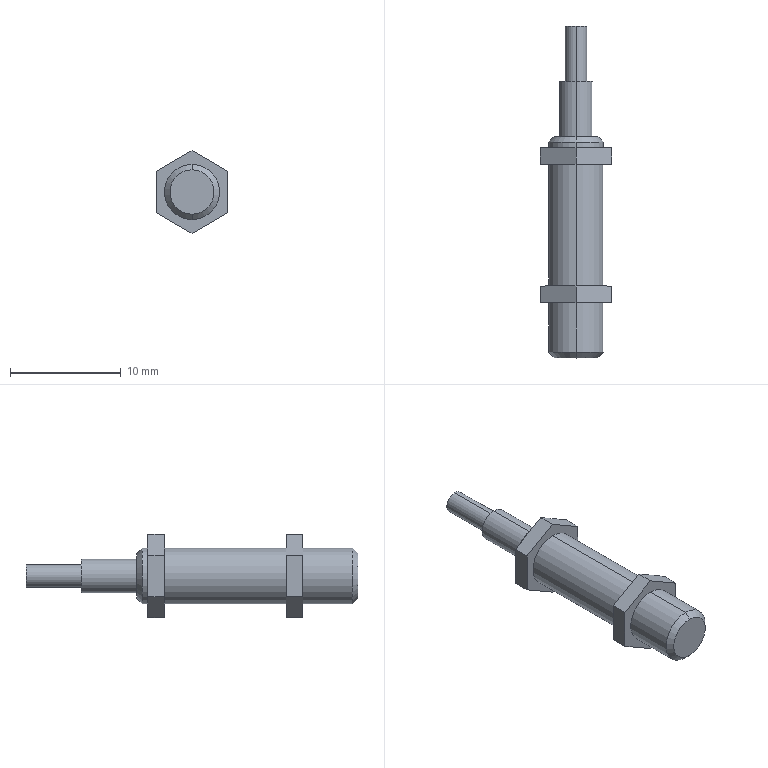Part | STEP file | Guide wheel mechanism revised.sldasm-Part-49 | 1 solid | 34 faces | box 6.5 x 30 x 7.506 mm | volume 490.949 mm3 | plane 20 | cylinder 10 | cone 4 | commonest cylinder face diameters 5 x6 2 x2 3 x2
STEP:
#1=CARTESIAN_POINT('',(0.,17.5,-2.5));
#2=VERTEX_POINT('',#1);
#3=CARTESIAN_POINT('',(0.,17.5,2.5));
#4=VERTEX_POINT('',#3);
#5=CARTESIAN_POINT('',(0.,17.5,0.));
#6=DIRECTION('',(0.,-1.,0.));
#7=DIRECTION('',(0.,0.,-1.));
#8=AXIS2_PLACEMENT_3D('',#5,#6,#7);
#9=CIRCLE('',#8,2.5);
#10=EDGE_CURVE('',#2,#4,#9,.T.);
#11=ORIENTED_EDGE('',*,*,#10,.T.);
#12=CARTESIAN_POINT('',(0.,6.5,2.5));
#13=VERTEX_POINT('',#12);
#14=CARTESIAN_POINT('',(0.,20.,2.5));
#15=DIRECTION('',(0.,-1.,0.));
#16=VECTOR('',#15,1000.);
#17=LINE('',#14,#16);
#18=EDGE_CURVE('',#4,#13,#17,.T.);
#19=ORIENTED_EDGE('',*,*,#18,.T.);
#20=CARTESIAN_POINT('',(0.,6.5,-2.5));
#21=VERTEX_POINT('',#20);
#22=CARTESIAN_POINT('',(0.,6.5,0.));
#23=DIRECTION('',(0.,-1.,0.));
#24=DIRECTION('',(0.,0.,-1.));
#25=AXIS2_PLACEMENT_3D('',#22,#23,#24);
#26=CIRCLE('',#25,2.5);
#27=EDGE_CURVE('',#21,#13,#26,.T.);
#28=ORIENTED_EDGE('',*,*,#27,.F.);
#29=CARTESIAN_POINT('',(0.,20.,-2.5));
#30=DIRECTION('',(0.,-1.,0.));
#31=VECTOR('',#30,1000.);
#32=LINE('',#29,#31);
#33=EDGE_CURVE('',#2,#21,#32,.T.);
#34=ORIENTED_EDGE('',*,*,#33,.F.);
#35=EDGE_LOOP('',(#11,#19,#28,#34));
#36=FACE_OUTER_BOUND('',#35,.T.);
#37=CARTESIAN_POINT('',(0.,20.,0.));
#38=DIRECTION('',(0.,-1.,0.));
#39=DIRECTION('',(0.,0.,-1.));
#40=AXIS2_PLACEMENT_3D('',#37,#38,#39);
#41=CYLINDRICAL_SURFACE('',#40,2.5);
#42=ADVANCED_FACE('',(#36),#41,.T.);
#43=CARTESIAN_POINT('',(0.,5.,-2.5));
#44=VERTEX_POINT('',#43);
#45=CARTESIAN_POINT('',(0.,5.,2.5));
#46=VERTEX_POINT('',#45);
#47=CARTESIAN_POINT('',(0.,5.,0.));
#48=DIRECTION('',(0.,-1.,0.));
#49=DIRECTION('',(0.,0.,-1.));
#50=AXIS2_PLACEMENT_3D('',#47,#48,#49);
#51=CIRCLE('',#50,2.5);
#52=EDGE_CURVE('',#44,#46,#51,.T.);
#53=ORIENTED_EDGE('',*,*,#52,.T.);
#54=CARTESIAN_POINT('',(0.,0.5,2.5));
#55=VERTEX_POINT('',#54);
#56=CARTESIAN_POINT('',(0.,20.,2.5));
#57=DIRECTION('',(0.,-1.,0.));
#58=VECTOR('',#57,1000.);
#59=LINE('',#56,#58);
#60=EDGE_CURVE('',#46,#55,#59,.T.);
#61=ORIENTED_EDGE('',*,*,#60,.T.);
#62=CARTESIAN_POINT('',(0.,0.5,-2.5));
#63=VERTEX_POINT('',#62);
#64=CARTESIAN_POINT('',(0.,0.5,0.));
#65=DIRECTION('',(0.,1.,0.));
#66=DIRECTION('',(0.,0.,1.));
#67=AXIS2_PLACEMENT_3D('',#64,#65,#66);
#68=CIRCLE('',#67,2.5);
#69=EDGE_CURVE('',#55,#63,#68,.T.);
#70=ORIENTED_EDGE('',*,*,#69,.T.);
#71=CARTESIAN_POINT('',(0.,20.,-2.5));
#72=DIRECTION('',(0.,-1.,0.));
#73=VECTOR('',#72,1000.);
#74=LINE('',#71,#73);
#75=EDGE_CURVE('',#44,#63,#74,.T.);
#76=ORIENTED_EDGE('',*,*,#75,.F.);
#77=EDGE_LOOP('',(#53,#61,#70,#76));
#78=FACE_OUTER_BOUND('',#77,.T.);
#79=CARTESIAN_POINT('',(0.,20.,0.));
#80=DIRECTION('',(0.,-1.,0.));
#81=DIRECTION('',(0.,0.,-1.));
#82=AXIS2_PLACEMENT_3D('',#79,#80,#81);
#83=CYLINDRICAL_SURFACE('',#82,2.5);
#84=ADVANCED_FACE('',(#78),#83,.T.);
#85=CARTESIAN_POINT('',(0.,0.,-2.));
#86=VERTEX_POINT('',#85);
#87=CARTESIAN_POINT('',(0.,0.,2.));
#88=VERTEX_POINT('',#87);
#89=CARTESIAN_POINT('',(0.,0.,0.));
#90=DIRECTION('',(0.,-1.,0.));
#91=DIRECTION('',(0.,0.,1.));
#92=AXIS2_PLACEMENT_3D('',#89,#90,#91);
#93=CIRCLE('',#92,2.);
#94=EDGE_CURVE('',#86,#88,#93,.T.);
#95=ORIENTED_EDGE('',*,*,#94,.F.);
#96=CARTESIAN_POINT('',(0.,0.5,-2.5));
#97=DIRECTION('',(0.,0.7071,-0.7071));
#98=VECTOR('',#97,1000.);
#99=LINE('',#96,#98);
#100=EDGE_CURVE('',#86,#63,#99,.T.);
#101=ORIENTED_EDGE('',*,*,#100,.T.);
#102=ORIENTED_EDGE('',*,*,#69,.F.);
#103=CARTESIAN_POINT('',(0.,0.5,2.5));
#104=DIRECTION('',(0.,0.7071,0.7071));
#105=VECTOR('',#104,1000.);
#106=LINE('',#103,#105);
#107=EDGE_CURVE('',#88,#55,#106,.T.);
#108=ORIENTED_EDGE('',*,*,#107,.F.);
#109=EDGE_LOOP('',(#95,#101,#102,#108));
#110=FACE_OUTER_BOUND('',#109,.T.);
#111=CARTESIAN_POINT('',(0.,0.5,0.));
#112=DIRECTION('',(0.,1.,0.));
#113=DIRECTION('',(0.,0.,1.));
#114=AXIS2_PLACEMENT_3D('',#111,#112,#113);
#115=CONICAL_SURFACE('',#114,2.5,0.7854);
#116=ADVANCED_FACE('',(#110),#115,.T.);
#117=CARTESIAN_POINT('',(0.,30.,1.));
#118=VERTEX_POINT('',#117);
#119=CARTESIAN_POINT('',(0.,30.,-1.));
#120=VERTEX_POINT('',#119);
#121=CARTESIAN_POINT('',(0.,30.,0.));
#122=DIRECTION('',(0.,1.,0.));
#123=DIRECTION('',(0.,0.,1.));
#124=AXIS2_PLACEMENT_3D('',#121,#122,#123);
#125=CIRCLE('',#124,1.);
#126=EDGE_CURVE('',#118,#120,#125,.T.);
#127=ORIENTED_EDGE('',*,*,#126,.F.);
#128=CARTESIAN_POINT('',(0.,25.,1.));
#129=VERTEX_POINT('',#128);
#130=CARTESIAN_POINT('',(0.,30.,1.));
#131=DIRECTION('',(0.,-1.,0.));
#132=VECTOR('',#131,1000.);
#133=LINE('',#130,#132);
#134=EDGE_CURVE('',#118,#129,#133,.T.);
#135=ORIENTED_EDGE('',*,*,#134,.T.);
#136=CARTESIAN_POINT('',(0.,25.,-1.));
#137=VERTEX_POINT('',#136);
#138=CARTESIAN_POINT('',(0.,25.,0.));
#139=DIRECTION('',(0.,1.,0.));
#140=DIRECTION('',(0.,0.,1.));
#141=AXIS2_PLACEMENT_3D('',#138,#139,#140);
#142=CIRCLE('',#141,1.);
#143=EDGE_CURVE('',#129,#137,#142,.T.);
#144=ORIENTED_EDGE('',*,*,#143,.T.);
#145=CARTESIAN_POINT('',(0.,30.,-1.));
#146=DIRECTION('',(0.,-1.,0.));
#147=VECTOR('',#146,1000.);
#148=LINE('',#145,#147);
#149=EDGE_CURVE('',#120,#137,#148,.T.);
#150=ORIENTED_EDGE('',*,*,#149,.F.);
#151=EDGE_LOOP('',(#127,#135,#144,#150));
#152=FACE_OUTER_BOUND('',#151,.T.);
#153=CARTESIAN_POINT('',(0.,30.,0.));
#154=DIRECTION('',(0.,-1.,0.));
#155=DIRECTION('',(0.,0.,-1.));
#156=AXIS2_PLACEMENT_3D('',#153,#154,#155);
#157=CYLINDRICAL_SURFACE('',#156,1.);
#158=ADVANCED_FACE('',(#152),#157,.T.);
#159=CARTESIAN_POINT('',(0.,25.,1.5));
#160=VERTEX_POINT('',#159);
#161=CARTESIAN_POINT('',(0.,25.,-1.5));
#162=VERTEX_POINT('',#161);
#163=CARTESIAN_POINT('',(0.,25.,0.));
#164=DIRECTION('',(0.,1.,0.));
#165=DIRECTION('',(0.,0.,1.));
#166=AXIS2_PLACEMENT_3D('',#163,#164,#165);
#167=CIRCLE('',#166,1.5);
#168=EDGE_CURVE('',#160,#162,#167,.T.);
#169=ORIENTED_EDGE('',*,*,#168,.F.);
#170=CARTESIAN_POINT('',(0.,20.,1.5));
#171=VERTEX_POINT('',#170);
#172=CARTESIAN_POINT('',(0.,25.,1.5));
#173=DIRECTION('',(0.,-1.,0.));
#174=VECTOR('',#173,1000.);
#175=LINE('',#172,#174);
#176=EDGE_CURVE('',#160,#171,#175,.T.);
#177=ORIENTED_EDGE('',*,*,#176,.T.);
#178=CARTESIAN_POINT('',(0.,20.,-1.5));
#179=VERTEX_POINT('',#178);
#180=CARTESIAN_POINT('',(0.,20.,0.));
#181=DIRECTION('',(0.,1.,0.));
#182=DIRECTION('',(0.,0.,1.));
#183=AXIS2_PLACEMENT_3D('',#180,#181,#182);
#184=CIRCLE('',#183,1.5);
#185=EDGE_CURVE('',#171,#179,#184,.T.);
#186=ORIENTED_EDGE('',*,*,#185,.T.);
#187=CARTESIAN_POINT('',(0.,25.,-1.5));
#188=DIRECTION('',(0.,-1.,0.));
#189=VECTOR('',#188,1000.);
#190=LINE('',#187,#189);
#191=EDGE_CURVE('',#162,#179,#190,.T.);
#192=ORIENTED_EDGE('',*,*,#191,.F.);
#193=EDGE_LOOP('',(#169,#177,#186,#192));
#194=FACE_OUTER_BOUND('',#193,.T.);
#195=CARTESIAN_POINT('',(0.,25.,0.));
#196=DIRECTION('',(0.,-1.,0.));
#197=DIRECTION('',(0.,0.,-1.));
#198=AXIS2_PLACEMENT_3D('',#195,#196,#197);
#199=CYLINDRICAL_SURFACE('',#198,1.5);
#200=ADVANCED_FACE('',(#194),#199,.T.);
#201=CARTESIAN_POINT('',(0.,20.,2.));
#202=VERTEX_POINT('',#201);
#203=CARTESIAN_POINT('',(0.,20.,-2.));
#204=VERTEX_POINT('',#203);
#205=CARTESIAN_POINT('',(0.,20.,0.));
#206=DIRECTION('',(0.,1.,0.));
#207=DIRECTION('',(0.,0.,1.));
#208=AXIS2_PLACEMENT_3D('',#205,#206,#207);
#209=CIRCLE('',#208,2.);
#210=EDGE_CURVE('',#202,#204,#209,.T.);
#211=ORIENTED_EDGE('',*,*,#210,.F.);
#212=CARTESIAN_POINT('',(0.,19.5,2.5));
#213=VERTEX_POINT('',#212);
#214=CARTESIAN_POINT('',(0.,20.,2.));
#215=DIRECTION('',(0.,-0.7071,0.7071));
#216=VECTOR('',#215,1000.);
#217=LINE('',#214,#216);
#218=EDGE_CURVE('',#202,#213,#217,.T.);
#219=ORIENTED_EDGE('',*,*,#218,.T.);
#220=CARTESIAN_POINT('',(0.,19.5,-2.5));
#221=VERTEX_POINT('',#220);
#222=CARTESIAN_POINT('',(0.,19.5,0.));
#223=DIRECTION('',(0.,-1.,0.));
#224=DIRECTION('',(0.,0.,1.));
#225=AXIS2_PLACEMENT_3D('',#222,#223,#224);
#226=CIRCLE('',#225,2.5);
#227=EDGE_CURVE('',#221,#213,#226,.T.);
#228=ORIENTED_EDGE('',*,*,#227,.F.);
#229=CARTESIAN_POINT('',(0.,20.,-2.));
#230=DIRECTION('',(0.,-0.7071,-0.7071));
#231=VECTOR('',#230,1000.);
#232=LINE('',#229,#231);
#233=EDGE_CURVE('',#204,#221,#232,.T.);
#234=ORIENTED_EDGE('',*,*,#233,.F.);
#235=EDGE_LOOP('',(#211,#219,#228,#234));
#236=FACE_OUTER_BOUND('',#235,.T.);
#237=CARTESIAN_POINT('',(0.,20.,0.));
#238=DIRECTION('',(0.,-1.,0.));
#239=DIRECTION('',(0.,0.,-1.));
#240=AXIS2_PLACEMENT_3D('',#237,#238,#239);
#241=CONICAL_SURFACE('',#240,2.,0.7854);
#242=ADVANCED_FACE('',(#236),#241,.T.);
#243=ORIENTED_EDGE('',*,*,#227,.T.);
#244=CARTESIAN_POINT('',(0.,19.,2.5));
#245=VERTEX_POINT('',#244);
#246=CARTESIAN_POINT('',(0.,20.,2.5));
#247=DIRECTION('',(0.,-1.,0.));
#248=VECTOR('',#247,1000.);
#249=LINE('',#246,#248);
#250=EDGE_CURVE('',#213,#245,#249,.T.);
#251=ORIENTED_EDGE('',*,*,#250,.T.);
#252=CARTESIAN_POINT('',(0.,19.,-2.5));
#253=VERTEX_POINT('',#252);
#254=CARTESIAN_POINT('',(0.,19.,0.));
#255=DIRECTION('',(0.,-1.,0.));
#256=DIRECTION('',(0.,0.,-1.));
#257=AXIS2_PLACEMENT_3D('',#254,#255,#256);
#258=CIRCLE('',#257,2.5);
#259=EDGE_CURVE('',#253,#245,#258,.T.);
#260=ORIENTED_EDGE('',*,*,#259,.F.);
#261=CARTESIAN_POINT('',(0.,20.,-2.5));
#262=DIRECTION('',(0.,-1.,0.));
#263=VECTOR('',#262,1000.);
#264=LINE('',#261,#263);
#265=EDGE_CURVE('',#221,#253,#264,.T.);
#266=ORIENTED_EDGE('',*,*,#265,.F.);
#267=EDGE_LOOP('',(#243,#251,#260,#266));
#268=FACE_OUTER_BOUND('',#267,.T.);
#269=CARTESIAN_POINT('',(0.,20.,0.));
#270=DIRECTION('',(0.,-1.,0.));
#271=DIRECTION('',(0.,0.,-1.));
#272=AXIS2_PLACEMENT_3D('',#269,#270,#271);
#273=CYLINDRICAL_SURFACE('',#272,2.5);
#274=ADVANCED_FACE('',(#268),#273,.T.);
#275=ORIENTED_EDGE('',*,*,#250,.F.);
#276=CARTESIAN_POINT('',(0.,19.5,0.));
#277=DIRECTION('',(0.,-1.,0.));
#278=DIRECTION('',(0.,0.,1.));
#279=AXIS2_PLACEMENT_3D('',#276,#277,#278);
#280=CIRCLE('',#279,2.5);
#281=EDGE_CURVE('',#213,#221,#280,.T.);
#282=ORIENTED_EDGE('',*,*,#281,.T.);
#283=ORIENTED_EDGE('',*,*,#265,.T.);
#284=CARTESIAN_POINT('',(0.,19.,0.));
#285=DIRECTION('',(0.,-1.,0.));
#286=DIRECTION('',(0.,0.,-1.));
#287=AXIS2_PLACEMENT_3D('',#284,#285,#286);
#288=CIRCLE('',#287,2.5);
#289=EDGE_CURVE('',#245,#253,#288,.T.);
#290=ORIENTED_EDGE('',*,*,#289,.F.);
#291=EDGE_LOOP('',(#275,#282,#283,#290));
#292=FACE_OUTER_BOUND('',#291,.T.);
#293=CARTESIAN_POINT('',(0.,20.,0.));
#294=DIRECTION('',(0.,-1.,0.));
#295=DIRECTION('',(0.,0.,-1.));
#296=AXIS2_PLACEMENT_3D('',#293,#294,#295);
#297=CYLINDRICAL_SURFACE('',#296,2.5);
#298=ADVANCED_FACE('',(#292),#297,.T.);
#299=CARTESIAN_POINT('',(0.,25.,0.));
#300=DIRECTION('',(0.,1.,0.));
#301=DIRECTION('',(0.,0.,1.));
#302=AXIS2_PLACEMENT_3D('',#299,#300,#301);
#303=CIRCLE('',#302,1.5);
#304=EDGE_CURVE('',#162,#160,#303,.T.);
#305=ORIENTED_EDGE('',*,*,#304,.T.);
#306=ORIENTED_EDGE('',*,*,#168,.T.);
#307=EDGE_LOOP('',(#305,#306));
#308=FACE_OUTER_BOUND('',#307,.T.);
#309=CARTESIAN_POINT('',(0.,25.,0.));
#310=DIRECTION('',(0.,1.,0.));
#311=DIRECTION('',(0.,0.,1.));
#312=AXIS2_PLACEMENT_3D('',#309,#310,#311);
#313=CIRCLE('',#312,1.);
#314=EDGE_CURVE('',#137,#129,#313,.T.);
#315=ORIENTED_EDGE('',*,*,#314,.F.);
#316=ORIENTED_EDGE('',*,*,#143,.F.);
#317=EDGE_LOOP('',(#315,#316));
#318=FACE_BOUND('',#317,.T.);
#319=CARTESIAN_POINT('',(0.,25.,0.));
#320=DIRECTION('',(0.,1.,0.));
#321=DIRECTION('',(0.,0.,1.));
#322=AXIS2_PLACEMENT_3D('',#319,#320,#321);
#323=PLANE('',#322);
#324=ADVANCED_FACE('',(#308,#318),#323,.T.);
#325=CARTESIAN_POINT('',(0.,20.,0.));
#326=DIRECTION('',(0.,1.,0.));
#327=DIRECTION('',(0.,0.,1.));
#328=AXIS2_PLACEMENT_3D('',#325,#326,#327);
#329=CIRCLE('',#328,2.);
#330=EDGE_CURVE('',#204,#202,#329,.T.);
#331=ORIENTED_EDGE('',*,*,#330,.T.);
#332=ORIENTED_EDGE('',*,*,#210,.T.);
#333=EDGE_LOOP('',(#331,#332));
#334=FACE_OUTER_BOUND('',#333,.T.);
#335=CARTESIAN_POINT('',(0.,20.,0.));
#336=DIRECTION('',(0.,1.,0.));
#337=DIRECTION('',(0.,0.,1.));
#338=AXIS2_PLACEMENT_3D('',#335,#336,#337);
#339=CIRCLE('',#338,1.5);
#340=EDGE_CURVE('',#179,#171,#339,.T.);
#341=ORIENTED_EDGE('',*,*,#340,.F.);
#342=ORIENTED_EDGE('',*,*,#185,.F.);
#343=EDGE_LOOP('',(#341,#342));
#344=FACE_BOUND('',#343,.T.);
#345=CARTESIAN_POINT('',(0.,20.,0.));
#346=DIRECTION('',(0.,1.,0.));
#347=DIRECTION('',(0.,0.,1.));
#348=AXIS2_PLACEMENT_3D('',#345,#346,#347);
#349=PLANE('',#348);
#350=ADVANCED_FACE('',(#334,#344),#349,.T.);
#351=ORIENTED_EDGE('',*,*,#218,.F.);
#352=ORIENTED_EDGE('',*,*,#330,.F.);
#353=ORIENTED_EDGE('',*,*,#233,.T.);
#354=ORIENTED_EDGE('',*,*,#281,.F.);
#355=EDGE_LOOP('',(#351,#352,#353,#354));
#356=FACE_OUTER_BOUND('',#355,.T.);
#357=CARTESIAN_POINT('',(0.,20.,0.));
#358=DIRECTION('',(0.,-1.,0.));
#359=DIRECTION('',(0.,0.,-1.));
#360=AXIS2_PLACEMENT_3D('',#357,#358,#359);
#361=CONICAL_SURFACE('',#360,2.,0.7854);
#362=ADVANCED_FACE('',(#356),#361,.T.);
#363=ORIENTED_EDGE('',*,*,#176,.F.);
#364=ORIENTED_EDGE('',*,*,#304,.F.);
#365=ORIENTED_EDGE('',*,*,#191,.T.);
#366=ORIENTED_EDGE('',*,*,#340,.T.);
#367=EDGE_LOOP('',(#363,#364,#365,#366));
#368=FACE_OUTER_BOUND('',#367,.T.);
#369=CARTESIAN_POINT('',(0.,25.,0.));
#370=DIRECTION('',(0.,-1.,0.));
#371=DIRECTION('',(0.,0.,-1.));
#372=AXIS2_PLACEMENT_3D('',#369,#370,#371);
#373=CYLINDRICAL_SURFACE('',#372,1.5);
#374=ADVANCED_FACE('',(#368),#373,.T.);
#375=ORIENTED_EDGE('',*,*,#134,.F.);
#376=CARTESIAN_POINT('',(0.,30.,0.));
#377=DIRECTION('',(0.,1.,0.));
#378=DIRECTION('',(0.,0.,1.));
#379=AXIS2_PLACEMENT_3D('',#376,#377,#378);
#380=CIRCLE('',#379,1.);
#381=EDGE_CURVE('',#120,#118,#380,.T.);
#382=ORIENTED_EDGE('',*,*,#381,.F.);
#383=ORIENTED_EDGE('',*,*,#149,.T.);
#384=ORIENTED_EDGE('',*,*,#314,.T.);
#385=EDGE_LOOP('',(#375,#382,#383,#384));
#386=FACE_OUTER_BOUND('',#385,.T.);
#387=CARTESIAN_POINT('',(0.,30.,0.));
#388=DIRECTION('',(0.,-1.,0.));
#389=DIRECTION('',(0.,0.,-1.));
#390=AXIS2_PLACEMENT_3D('',#387,#388,#389);
#391=CYLINDRICAL_SURFACE('',#390,1.);
#392=ADVANCED_FACE('',(#386),#391,.T.);
#393=ORIENTED_EDGE('',*,*,#381,.T.);
#394=ORIENTED_EDGE('',*,*,#126,.T.);
#395=EDGE_LOOP('',(#393,#394));
#396=FACE_OUTER_BOUND('',#395,.T.);
#397=CARTESIAN_POINT('',(0.,30.,0.));
#398=DIRECTION('',(0.,1.,0.));
#399=DIRECTION('',(0.,0.,1.));
#400=AXIS2_PLACEMENT_3D('',#397,#398,#399);
#401=PLANE('',#400);
#402=ADVANCED_FACE('',(#396),#401,.T.);
#403=CARTESIAN_POINT('',(3.25,17.5,1.876));
#404=VERTEX_POINT('',#403);
#405=CARTESIAN_POINT('',(0.,17.5,3.753));
#406=VERTEX_POINT('',#405);
#407=CARTESIAN_POINT('',(3.25,17.5,1.876));
#408=DIRECTION('',(-0.866,0.,0.5));
#409=VECTOR('',#408,1000.);
#410=LINE('',#407,#409);
#411=EDGE_CURVE('',#404,#406,#410,.T.);
#412=ORIENTED_EDGE('',*,*,#411,.F.);
#413=CARTESIAN_POINT('',(3.25,19.,1.876));
#414=VERTEX_POINT('',#413);
#415=CARTESIAN_POINT('',(3.25,19.,1.876));
#416=DIRECTION('',(0.,-1.,0.));
#417=VECTOR('',#416,1000.);
#418=LINE('',#415,#417);
#419=EDGE_CURVE('',#414,#404,#418,.T.);
#420=ORIENTED_EDGE('',*,*,#419,.F.);
#421=CARTESIAN_POINT('',(0.,19.,3.753));
#422=VERTEX_POINT('',#421);
#423=CARTESIAN_POINT('',(3.25,19.,1.876));
#424=DIRECTION('',(-0.866,0.,0.5));
#425=VECTOR('',#424,1000.);
#426=LINE('',#423,#425);
#427=EDGE_CURVE('',#414,#422,#426,.T.);
#428=ORIENTED_EDGE('',*,*,#427,.T.);
#429=CARTESIAN_POINT('',(0.,19.,3.753));
#430=DIRECTION('',(0.,-1.,0.));
#431=VECTOR('',#430,1000.);
#432=LINE('',#429,#431);
#433=EDGE_CURVE('',#422,#406,#432,.T.);
#434=ORIENTED_EDGE('',*,*,#433,.T.);
#435=EDGE_LOOP('',(#412,#420,#428,#434));
#436=FACE_OUTER_BOUND('',#435,.T.);
#437=CARTESIAN_POINT('',(3.25,19.,1.876));
#438=DIRECTION('',(0.5,0.,0.866));
#439=DIRECTION('',(0.866,0.,-0.5));
#440=AXIS2_PLACEMENT_3D('',#437,#438,#439);
#441=PLANE('',#440);
#442=ADVANCED_FACE('',(#436),#441,.T.);
#443=CARTESIAN_POINT('',(3.25,17.5,-1.876));
#444=VERTEX_POINT('',#443);
#445=CARTESIAN_POINT('',(3.25,17.5,-1.876));
#446=DIRECTION('',(0.,0.,1.));
#447=VECTOR('',#446,1000.);
#448=LINE('',#445,#447);
#449=EDGE_CURVE('',#444,#404,#448,.T.);
#450=ORIENTED_EDGE('',*,*,#449,.F.);
#451=CARTESIAN_POINT('',(3.25,19.,-1.876));
#452=VERTEX_POINT('',#451);
#453=CARTESIAN_POINT('',(3.25,19.,-1.876));
#454=DIRECTION('',(0.,-1.,0.));
#455=VECTOR('',#454,1000.);
#456=LINE('',#453,#455);
#457=EDGE_CURVE('',#452,#444,#456,.T.);
#458=ORIENTED_EDGE('',*,*,#457,.F.);
#459=CARTESIAN_POINT('',(3.25,19.,-1.876));
#460=DIRECTION('',(0.,0.,1.));
#461=VECTOR('',#460,1000.);
#462=LINE('',#459,#461);
#463=EDGE_CURVE('',#452,#414,#462,.T.);
#464=ORIENTED_EDGE('',*,*,#463,.T.);
#465=ORIENTED_EDGE('',*,*,#419,.T.);
#466=EDGE_LOOP('',(#450,#458,#464,#465));
#467=FACE_OUTER_BOUND('',#466,.T.);
#468=CARTESIAN_POINT('',(3.25,19.,-1.876));
#469=DIRECTION('',(1.,0.,0.));
#470=DIRECTION('',(0.,0.,-1.));
#471=AXIS2_PLACEMENT_3D('',#468,#469,#470);
#472=PLANE('',#471);
#473=ADVANCED_FACE('',(#467),#472,.T.);
#474=CARTESIAN_POINT('',(0.,17.5,-3.753));
#475=VERTEX_POINT('',#474);
#476=CARTESIAN_POINT('',(0.,17.5,-3.753));
#477=DIRECTION('',(0.866,0.,0.5));
#478=VECTOR('',#477,1000.);
#479=LINE('',#476,#478);
#480=EDGE_CURVE('',#475,#444,#479,.T.);
#481=ORIENTED_EDGE('',*,*,#480,.F.);
#482=CARTESIAN_POINT('',(0.,19.,-3.753));
#483=VERTEX_POINT('',#482);
#484=CARTESIAN_POINT('',(0.,19.,-3.753));
#485=DIRECTION('',(0.,-1.,0.));
#486=VECTOR('',#485,1000.);
#487=LINE('',#484,#486);
#488=EDGE_CURVE('',#483,#475,#487,.T.);
#489=ORIENTED_EDGE('',*,*,#488,.F.);
#490=CARTESIAN_POINT('',(0.,19.,-3.753));
#491=DIRECTION('',(0.866,0.,0.5));
#492=VECTOR('',#491,1000.);
#493=LINE('',#490,#492);
#494=EDGE_CURVE('',#483,#452,#493,.T.);
#495=ORIENTED_EDGE('',*,*,#494,.T.);
#496=ORIENTED_EDGE('',*,*,#457,.T.);
#497=EDGE_LOOP('',(#481,#489,#495,#496));
#498=FACE_OUTER_BOUND('',#497,.T.);
#499=CARTESIAN_POINT('',(0.,19.,-3.753));
#500=DIRECTION('',(0.5,0.,-0.866));
#501=DIRECTION('',(-0.866,0.,-0.5));
#502=AXIS2_PLACEMENT_3D('',#499,#500,#501);
#503=PLANE('',#502);
#504=ADVANCED_FACE('',(#498),#503,.T.);
#505=CARTESIAN_POINT('',(-3.25,17.5,-1.876));
#506=VERTEX_POINT('',#505);
#507=CARTESIAN_POINT('',(-3.25,17.5,-1.876));
#508=DIRECTION('',(0.866,0.,-0.5));
#509=VECTOR('',#508,1000.);
#510=LINE('',#507,#509);
#511=EDGE_CURVE('',#506,#475,#510,.T.);
#512=ORIENTED_EDGE('',*,*,#511,.F.);
#513=CARTESIAN_POINT('',(-3.25,19.,-1.876));
#514=VERTEX_POINT('',#513);
#515=CARTESIAN_POINT('',(-3.25,19.,-1.876));
#516=DIRECTION('',(0.,-1.,0.));
#517=VECTOR('',#516,1000.);
#518=LINE('',#515,#517);
#519=EDGE_CURVE('',#514,#506,#518,.T.);
#520=ORIENTED_EDGE('',*,*,#519,.F.);
#521=CARTESIAN_POINT('',(-3.25,19.,-1.876));
#522=DIRECTION('',(0.866,0.,-0.5));
#523=VECTOR('',#522,1000.);
#524=LINE('',#521,#523);
#525=EDGE_CURVE('',#514,#483,#524,.T.);
#526=ORIENTED_EDGE('',*,*,#525,.T.);
#527=ORIENTED_EDGE('',*,*,#488,.T.);
#528=EDGE_LOOP('',(#512,#520,#526,#527));
#529=FACE_OUTER_BOUND('',#528,.T.);
#530=CARTESIAN_POINT('',(-3.25,19.,-1.876));
#531=DIRECTION('',(-0.5,0.,-0.866));
#532=DIRECTION('',(-0.866,0.,0.5));
#533=AXIS2_PLACEMENT_3D('',#530,#531,#532);
#534=PLANE('',#533);
#535=ADVANCED_FACE('',(#529),#534,.T.);
#536=CARTESIAN_POINT('',(-3.25,17.5,1.876));
#537=VERTEX_POINT('',#536);
#538=CARTESIAN_POINT('',(-3.25,17.5,1.876));
#539=DIRECTION('',(0.,0.,-1.));
#540=VECTOR('',#539,1000.);
#541=LINE('',#538,#540);
#542=EDGE_CURVE('',#537,#506,#541,.T.);
#543=ORIENTED_EDGE('',*,*,#542,.F.);
#544=CARTESIAN_POINT('',(-3.25,19.,1.876));
#545=VERTEX_POINT('',#544);
#546=CARTESIAN_POINT('',(-3.25,19.,1.876));
#547=DIRECTION('',(0.,-1.,0.));
#548=VECTOR('',#547,1000.);
#549=LINE('',#546,#548);
#550=EDGE_CURVE('',#545,#537,#549,.T.);
#551=ORIENTED_EDGE('',*,*,#550,.F.);
#552=CARTESIAN_POINT('',(-3.25,19.,1.876));
#553=DIRECTION('',(0.,0.,-1.));
#554=VECTOR('',#553,1000.);
#555=LINE('',#552,#554);
#556=EDGE_CURVE('',#545,#514,#555,.T.);
#557=ORIENTED_EDGE('',*,*,#556,.T.);
#558=ORIENTED_EDGE('',*,*,#519,.T.);
#559=EDGE_LOOP('',(#543,#551,#557,#558));
#560=FACE_OUTER_BOUND('',#559,.T.);
#561=CARTESIAN_POINT('',(-3.25,19.,1.876));
#562=DIRECTION('',(-1.,0.,0.));
#563=DIRECTION('',(0.,0.,1.));
#564=AXIS2_PLACEMENT_3D('',#561,#562,#563);
#565=PLANE('',#564);
#566=ADVANCED_FACE('',(#560),#565,.T.);
#567=CARTESIAN_POINT('',(0.,17.5,3.753));
#568=DIRECTION('',(-0.866,0.,-0.5));
#569=VECTOR('',#568,1000.);
#570=LINE('',#567,#569);
#571=EDGE_CURVE('',#406,#537,#570,.T.);
#572=ORIENTED_EDGE('',*,*,#571,.F.);
#573=ORIENTED_EDGE('',*,*,#433,.F.);
#574=CARTESIAN_POINT('',(0.,19.,3.753));
#575=DIRECTION('',(-0.866,0.,-0.5));
#576=VECTOR('',#575,1000.);
#577=LINE('',#574,#576);
#578=EDGE_CURVE('',#422,#545,#577,.T.);
#579=ORIENTED_EDGE('',*,*,#578,.T.);
#580=ORIENTED_EDGE('',*,*,#550,.T.);
#581=EDGE_LOOP('',(#572,#573,#579,#580));
#582=FACE_OUTER_BOUND('',#581,.T.);
#583=CARTESIAN_POINT('',(0.,19.,3.753));
#584=DIRECTION('',(-0.5,0.,0.866));
#585=DIRECTION('',(0.866,0.,0.5));
#586=AXIS2_PLACEMENT_3D('',#583,#584,#585);
#587=PLANE('',#586);
#588=ADVANCED_FACE('',(#582),#587,.T.);
#589=ORIENTED_EDGE('',*,*,#259,.T.);
#590=ORIENTED_EDGE('',*,*,#289,.T.);
#591=EDGE_LOOP('',(#589,#590));
#592=FACE_BOUND('',#591,.T.);
#593=ORIENTED_EDGE('',*,*,#427,.F.);
#594=ORIENTED_EDGE('',*,*,#463,.F.);
#595=ORIENTED_EDGE('',*,*,#494,.F.);
#596=ORIENTED_EDGE('',*,*,#525,.F.);
#597=ORIENTED_EDGE('',*,*,#556,.F.);
#598=ORIENTED_EDGE('',*,*,#578,.F.);
#599=EDGE_LOOP('',(#593,#594,#595,#596,#597,#598));
#600=FACE_OUTER_BOUND('',#599,.T.);
#601=CARTESIAN_POINT('',(0.,19.,0.));
#602=DIRECTION('',(0.,-1.,0.));
#603=DIRECTION('',(0.,0.,-1.));
#604=AXIS2_PLACEMENT_3D('',#601,#602,#603);
#605=PLANE('',#604);
#606=ADVANCED_FACE('',(#592,#600),#605,.F.);
#607=ORIENTED_EDGE('',*,*,#10,.F.);
#608=CARTESIAN_POINT('',(0.,17.5,0.));
#609=DIRECTION('',(0.,-1.,0.));
#610=DIRECTION('',(0.,0.,-1.));
#611=AXIS2_PLACEMENT_3D('',#608,#609,#610);
#612=CIRCLE('',#611,2.5);
#613=EDGE_CURVE('',#4,#2,#612,.T.);
#614=ORIENTED_EDGE('',*,*,#613,.F.);
#615=EDGE_LOOP('',(#607,#614));
#616=FACE_BOUND('',#615,.T.);
#617=ORIENTED_EDGE('',*,*,#411,.T.);
#618=ORIENTED_EDGE('',*,*,#571,.T.);
#619=ORIENTED_EDGE('',*,*,#542,.T.);
#620=ORIENTED_EDGE('',*,*,#511,.T.);
#621=ORIENTED_EDGE('',*,*,#480,.T.);
#622=ORIENTED_EDGE('',*,*,#449,.T.);
#623=EDGE_LOOP('',(#617,#618,#619,#620,#621,#622));
#624=FACE_OUTER_BOUND('',#623,.T.);
#625=CARTESIAN_POINT('',(0.,17.5,0.));
#626=DIRECTION('',(0.,-1.,0.));
#627=DIRECTION('',(0.,0.,-1.));
#628=AXIS2_PLACEMENT_3D('',#625,#626,#627);
#629=PLANE('',#628);
#630=ADVANCED_FACE('',(#616,#624),#629,.T.);
#631=CARTESIAN_POINT('',(0.,0.,0.));
#632=DIRECTION('',(0.,-1.,0.));
#633=DIRECTION('',(0.,0.,1.));
#634=AXIS2_PLACEMENT_3D('',#631,#632,#633);
#635=CIRCLE('',#634,2.);
#636=EDGE_CURVE('',#88,#86,#635,.T.);
#637=ORIENTED_EDGE('',*,*,#636,.T.);
#638=ORIENTED_EDGE('',*,*,#94,.T.);
#639=EDGE_LOOP('',(#637,#638));
#640=FACE_OUTER_BOUND('',#639,.T.);
#641=CARTESIAN_POINT('',(0.,0.,0.));
#642=DIRECTION('',(0.,1.,0.));
#643=DIRECTION('',(0.,0.,1.));
#644=AXIS2_PLACEMENT_3D('',#641,#642,#643);
#645=PLANE('',#644);
#646=ADVANCED_FACE('',(#640),#645,.F.);
#647=ORIENTED_EDGE('',*,*,#100,.F.);
#648=ORIENTED_EDGE('',*,*,#636,.F.);
#649=ORIENTED_EDGE('',*,*,#107,.T.);
#650=CARTESIAN_POINT('',(0.,0.5,0.));
#651=DIRECTION('',(0.,1.,0.));
#652=DIRECTION('',(0.,0.,1.));
#653=AXIS2_PLACEMENT_3D('',#650,#651,#652);
#654=CIRCLE('',#653,2.5);
#655=EDGE_CURVE('',#63,#55,#654,.T.);
#656=ORIENTED_EDGE('',*,*,#655,.F.);
#657=EDGE_LOOP('',(#647,#648,#649,#656));
#658=FACE_OUTER_BOUND('',#657,.T.);
#659=CARTESIAN_POINT('',(0.,0.5,0.));
#660=DIRECTION('',(0.,1.,0.));
#661=DIRECTION('',(0.,0.,1.));
#662=AXIS2_PLACEMENT_3D('',#659,#660,#661);
#663=CONICAL_SURFACE('',#662,2.5,0.7854);
#664=ADVANCED_FACE('',(#658),#663,.T.);
#665=ORIENTED_EDGE('',*,*,#60,.F.);
#666=CARTESIAN_POINT('',(0.,5.,0.));
#667=DIRECTION('',(0.,-1.,0.));
#668=DIRECTION('',(0.,0.,-1.));
#669=AXIS2_PLACEMENT_3D('',#666,#667,#668);
#670=CIRCLE('',#669,2.5);
#671=EDGE_CURVE('',#46,#44,#670,.T.);
#672=ORIENTED_EDGE('',*,*,#671,.T.);
#673=ORIENTED_EDGE('',*,*,#75,.T.);
#674=ORIENTED_EDGE('',*,*,#655,.T.);
#675=EDGE_LOOP('',(#665,#672,#673,#674));
#676=FACE_OUTER_BOUND('',#675,.T.);
#677=CARTESIAN_POINT('',(0.,20.,0.));
#678=DIRECTION('',(0.,-1.,0.));
#679=DIRECTION('',(0.,0.,-1.));
#680=AXIS2_PLACEMENT_3D('',#677,#678,#679);
#681=CYLINDRICAL_SURFACE('',#680,2.5);
#682=ADVANCED_FACE('',(#676),#681,.T.);
#683=ORIENTED_EDGE('',*,*,#52,.F.);
#684=ORIENTED_EDGE('',*,*,#671,.F.);
#685=EDGE_LOOP('',(#683,#684));
#686=FACE_BOUND('',#685,.T.);
#687=CARTESIAN_POINT('',(3.25,5.,1.876));
#688=VERTEX_POINT('',#687);
#689=CARTESIAN_POINT('',(0.,5.,3.753));
#690=VERTEX_POINT('',#689);
#691=CARTESIAN_POINT('',(3.25,5.,1.876));
#692=DIRECTION('',(-0.866,0.,0.5));
#693=VECTOR('',#692,1000.);
#694=LINE('',#691,#693);
#695=EDGE_CURVE('',#688,#690,#694,.T.);
#696=ORIENTED_EDGE('',*,*,#695,.T.);
#697=CARTESIAN_POINT('',(-3.25,5.,1.876));
#698=VERTEX_POINT('',#697);
#699=CARTESIAN_POINT('',(0.,5.,3.753));
#700=DIRECTION('',(-0.866,0.,-0.5));
#701=VECTOR('',#700,1000.);
#702=LINE('',#699,#701);
#703=EDGE_CURVE('',#690,#698,#702,.T.);
#704=ORIENTED_EDGE('',*,*,#703,.T.);
#705=CARTESIAN_POINT('',(-3.25,5.,-1.876));
#706=VERTEX_POINT('',#705);
#707=CARTESIAN_POINT('',(-3.25,5.,1.876));
#708=DIRECTION('',(0.,0.,-1.));
#709=VECTOR('',#708,1000.);
#710=LINE('',#707,#709);
#711=EDGE_CURVE('',#698,#706,#710,.T.);
#712=ORIENTED_EDGE('',*,*,#711,.T.);
#713=CARTESIAN_POINT('',(0.,5.,-3.753));
#714=VERTEX_POINT('',#713);
#715=CARTESIAN_POINT('',(-3.25,5.,-1.876));
#716=DIRECTION('',(0.866,0.,-0.5));
#717=VECTOR('',#716,1000.);
#718=LINE('',#715,#717);
#719=EDGE_CURVE('',#706,#714,#718,.T.);
#720=ORIENTED_EDGE('',*,*,#719,.T.);
#721=CARTESIAN_POINT('',(3.25,5.,-1.876));
#722=VERTEX_POINT('',#721);
#723=CARTESIAN_POINT('',(0.,5.,-3.753));
#724=DIRECTION('',(0.866,0.,0.5));
#725=VECTOR('',#724,1000.);
#726=LINE('',#723,#725);
#727=EDGE_CURVE('',#714,#722,#726,.T.);
#728=ORIENTED_EDGE('',*,*,#727,.T.);
#729=CARTESIAN_POINT('',(3.25,5.,-1.876));
#730=DIRECTION('',(0.,0.,1.));
#731=VECTOR('',#730,1000.);
#732=LINE('',#729,#731);
#733=EDGE_CURVE('',#722,#688,#732,.T.);
#734=ORIENTED_EDGE('',*,*,#733,.T.);
#735=EDGE_LOOP('',(#696,#704,#712,#720,#728,#734));
#736=FACE_OUTER_BOUND('',#735,.T.);
#737=CARTESIAN_POINT('',(0.,5.,0.));
#738=DIRECTION('',(0.,-1.,0.));
#739=DIRECTION('',(0.,0.,-1.));
#740=AXIS2_PLACEMENT_3D('',#737,#738,#739);
#741=PLANE('',#740);
#742=ADVANCED_FACE('',(#686,#736),#741,.T.);
#743=ORIENTED_EDGE('',*,*,#703,.F.);
#744=CARTESIAN_POINT('',(0.,6.5,3.753));
#745=VERTEX_POINT('',#744);
#746=CARTESIAN_POINT('',(0.,6.5,3.753));
#747=DIRECTION('',(0.,-1.,0.));
#748=VECTOR('',#747,1000.);
#749=LINE('',#746,#748);
#750=EDGE_CURVE('',#745,#690,#749,.T.);
#751=ORIENTED_EDGE('',*,*,#750,.F.);
#752=CARTESIAN_POINT('',(-3.25,6.5,1.876));
#753=VERTEX_POINT('',#752);
#754=CARTESIAN_POINT('',(0.,6.5,3.753));
#755=DIRECTION('',(-0.866,0.,-0.5));
#756=VECTOR('',#755,1000.);
#757=LINE('',#754,#756);
#758=EDGE_CURVE('',#745,#753,#757,.T.);
#759=ORIENTED_EDGE('',*,*,#758,.T.);
#760=CARTESIAN_POINT('',(-3.25,6.5,1.876));
#761=DIRECTION('',(0.,-1.,0.));
#762=VECTOR('',#761,1000.);
#763=LINE('',#760,#762);
#764=EDGE_CURVE('',#753,#698,#763,.T.);
#765=ORIENTED_EDGE('',*,*,#764,.T.);
#766=EDGE_LOOP('',(#743,#751,#759,#765));
#767=FACE_OUTER_BOUND('',#766,.T.);
#768=CARTESIAN_POINT('',(0.,6.5,3.753));
#769=DIRECTION('',(-0.5,0.,0.866));
#770=DIRECTION('',(0.866,0.,0.5));
#771=AXIS2_PLACEMENT_3D('',#768,#769,#770);
#772=PLANE('',#771);
#773=ADVANCED_FACE('',(#767),#772,.T.);
#774=ORIENTED_EDGE('',*,*,#711,.F.);
#775=ORIENTED_EDGE('',*,*,#764,.F.);
#776=CARTESIAN_POINT('',(-3.25,6.5,-1.876));
#777=VERTEX_POINT('',#776);
#778=CARTESIAN_POINT('',(-3.25,6.5,1.876));
#779=DIRECTION('',(0.,0.,-1.));
#780=VECTOR('',#779,1000.);
#781=LINE('',#778,#780);
#782=EDGE_CURVE('',#753,#777,#781,.T.);
#783=ORIENTED_EDGE('',*,*,#782,.T.);
#784=CARTESIAN_POINT('',(-3.25,6.5,-1.876));
#785=DIRECTION('',(0.,-1.,0.));
#786=VECTOR('',#785,1000.);
#787=LINE('',#784,#786);
#788=EDGE_CURVE('',#777,#706,#787,.T.);
#789=ORIENTED_EDGE('',*,*,#788,.T.);
#790=EDGE_LOOP('',(#774,#775,#783,#789));
#791=FACE_OUTER_BOUND('',#790,.T.);
#792=CARTESIAN_POINT('',(-3.25,6.5,1.876));
#793=DIRECTION('',(-1.,0.,0.));
#794=DIRECTION('',(0.,0.,1.));
#795=AXIS2_PLACEMENT_3D('',#792,#793,#794);
#796=PLANE('',#795);
#797=ADVANCED_FACE('',(#791),#796,.T.);
#798=ORIENTED_EDGE('',*,*,#719,.F.);
#799=ORIENTED_EDGE('',*,*,#788,.F.);
#800=CARTESIAN_POINT('',(0.,6.5,-3.753));
#801=VERTEX_POINT('',#800);
#802=CARTESIAN_POINT('',(-3.25,6.5,-1.876));
#803=DIRECTION('',(0.866,0.,-0.5));
#804=VECTOR('',#803,1000.);
#805=LINE('',#802,#804);
#806=EDGE_CURVE('',#777,#801,#805,.T.);
#807=ORIENTED_EDGE('',*,*,#806,.T.);
#808=CARTESIAN_POINT('',(0.,6.5,-3.753));
#809=DIRECTION('',(0.,-1.,0.));
#810=VECTOR('',#809,1000.);
#811=LINE('',#808,#810);
#812=EDGE_CURVE('',#801,#714,#811,.T.);
#813=ORIENTED_EDGE('',*,*,#812,.T.);
#814=EDGE_LOOP('',(#798,#799,#807,#813));
#815=FACE_OUTER_BOUND('',#814,.T.);
#816=CARTESIAN_POINT('',(-3.25,6.5,-1.876));
#817=DIRECTION('',(-0.5,0.,-0.866));
#818=DIRECTION('',(-0.866,0.,0.5));
#819=AXIS2_PLACEMENT_3D('',#816,#817,#818);
#820=PLANE('',#819);
#821=ADVANCED_FACE('',(#815),#820,.T.);
#822=ORIENTED_EDGE('',*,*,#727,.F.);
#823=ORIENTED_EDGE('',*,*,#812,.F.);
#824=CARTESIAN_POINT('',(3.25,6.5,-1.876));
#825=VERTEX_POINT('',#824);
#826=CARTESIAN_POINT('',(0.,6.5,-3.753));
#827=DIRECTION('',(0.866,0.,0.5));
#828=VECTOR('',#827,1000.);
#829=LINE('',#826,#828);
#830=EDGE_CURVE('',#801,#825,#829,.T.);
#831=ORIENTED_EDGE('',*,*,#830,.T.);
#832=CARTESIAN_POINT('',(3.25,6.5,-1.876));
#833=DIRECTION('',(0.,-1.,0.));
#834=VECTOR('',#833,1000.);
#835=LINE('',#832,#834);
#836=EDGE_CURVE('',#825,#722,#835,.T.);
#837=ORIENTED_EDGE('',*,*,#836,.T.);
#838=EDGE_LOOP('',(#822,#823,#831,#837));
#839=FACE_OUTER_BOUND('',#838,.T.);
#840=CARTESIAN_POINT('',(0.,6.5,-3.753));
#841=DIRECTION('',(0.5,0.,-0.866));
#842=DIRECTION('',(-0.866,0.,-0.5));
#843=AXIS2_PLACEMENT_3D('',#840,#841,#842);
#844=PLANE('',#843);
#845=ADVANCED_FACE('',(#839),#844,.T.);
#846=ORIENTED_EDGE('',*,*,#733,.F.);
#847=ORIENTED_EDGE('',*,*,#836,.F.);
#848=CARTESIAN_POINT('',(3.25,6.5,1.876));
#849=VERTEX_POINT('',#848);
#850=CARTESIAN_POINT('',(3.25,6.5,-1.876));
#851=DIRECTION('',(0.,0.,1.));
#852=VECTOR('',#851,1000.);
#853=LINE('',#850,#852);
#854=EDGE_CURVE('',#825,#849,#853,.T.);
#855=ORIENTED_EDGE('',*,*,#854,.T.);
#856=CARTESIAN_POINT('',(3.25,6.5,1.876));
#857=DIRECTION('',(0.,-1.,0.));
#858=VECTOR('',#857,1000.);
#859=LINE('',#856,#858);
#860=EDGE_CURVE('',#849,#688,#859,.T.);
#861=ORIENTED_EDGE('',*,*,#860,.T.);
#862=EDGE_LOOP('',(#846,#847,#855,#861));
#863=FACE_OUTER_BOUND('',#862,.T.);
#864=CARTESIAN_POINT('',(3.25,6.5,-1.876));
#865=DIRECTION('',(1.,0.,0.));
#866=DIRECTION('',(0.,0.,-1.));
#867=AXIS2_PLACEMENT_3D('',#864,#865,#866);
#868=PLANE('',#867);
#869=ADVANCED_FACE('',(#863),#868,.T.);
#870=ORIENTED_EDGE('',*,*,#695,.F.);
#871=ORIENTED_EDGE('',*,*,#860,.F.);
#872=CARTESIAN_POINT('',(3.25,6.5,1.876));
#873=DIRECTION('',(-0.866,0.,0.5));
#874=VECTOR('',#873,1000.);
#875=LINE('',#872,#874);
#876=EDGE_CURVE('',#849,#745,#875,.T.);
#877=ORIENTED_EDGE('',*,*,#876,.T.);
#878=ORIENTED_EDGE('',*,*,#750,.T.);
#879=EDGE_LOOP('',(#870,#871,#877,#878));
#880=FACE_OUTER_BOUND('',#879,.T.);
#881=CARTESIAN_POINT('',(3.25,6.5,1.876));
#882=DIRECTION('',(0.5,0.,0.866));
#883=DIRECTION('',(0.866,0.,-0.5));
#884=AXIS2_PLACEMENT_3D('',#881,#882,#883);
#885=PLANE('',#884);
#886=ADVANCED_FACE('',(#880),#885,.T.);
#887=ORIENTED_EDGE('',*,*,#27,.T.);
#888=CARTESIAN_POINT('',(0.,6.5,0.));
#889=DIRECTION('',(0.,-1.,0.));
#890=DIRECTION('',(0.,0.,-1.));
#891=AXIS2_PLACEMENT_3D('',#888,#889,#890);
#892=CIRCLE('',#891,2.5);
#893=EDGE_CURVE('',#13,#21,#892,.T.);
#894=ORIENTED_EDGE('',*,*,#893,.T.);
#895=EDGE_LOOP('',(#887,#894));
#896=FACE_BOUND('',#895,.T.);
#897=ORIENTED_EDGE('',*,*,#876,.F.);
#898=ORIENTED_EDGE('',*,*,#854,.F.);
#899=ORIENTED_EDGE('',*,*,#830,.F.);
#900=ORIENTED_EDGE('',*,*,#806,.F.);
#901=ORIENTED_EDGE('',*,*,#782,.F.);
#902=ORIENTED_EDGE('',*,*,#758,.F.);
#903=EDGE_LOOP('',(#897,#898,#899,#900,#901,#902));
#904=FACE_OUTER_BOUND('',#903,.T.);
#905=CARTESIAN_POINT('',(0.,6.5,0.));
#906=DIRECTION('',(0.,-1.,0.));
#907=DIRECTION('',(0.,0.,-1.));
#908=AXIS2_PLACEMENT_3D('',#905,#906,#907);
#909=PLANE('',#908);
#910=ADVANCED_FACE('',(#896,#904),#909,.F.);
#911=ORIENTED_EDGE('',*,*,#18,.F.);
#912=ORIENTED_EDGE('',*,*,#613,.T.);
#913=ORIENTED_EDGE('',*,*,#33,.T.);
#914=ORIENTED_EDGE('',*,*,#893,.F.);
#915=EDGE_LOOP('',(#911,#912,#913,#914));
#916=FACE_OUTER_BOUND('',#915,.T.);
#917=CARTESIAN_POINT('',(0.,20.,0.));
#918=DIRECTION('',(0.,-1.,0.));
#919=DIRECTION('',(0.,0.,-1.));
#920=AXIS2_PLACEMENT_3D('',#917,#918,#919);
#921=CYLINDRICAL_SURFACE('',#920,2.5);
#922=ADVANCED_FACE('',(#916),#921,.T.);
#923=CLOSED_SHELL('',(#42,#84,#116,#158,#200,#242,#274,#298,#324,#350,#362,#374,#392,#402,#442,#473,#504,#535,#566,#588,#606,#630,#646,#664,#682,#742,#773,#797,#821,#845,#869,#886,#910,#922));
#924=MANIFOLD_SOLID_BREP('',#923);
#925=CARTESIAN_POINT('',(0.,0.,0.));
#926=DIRECTION('',(0.,0.,1.));
#927=DIRECTION('',(1.,0.,0.));
#928=AXIS2_PLACEMENT_3D('',#925,#926,#927);
#929=(LENGTH_UNIT()NAMED_UNIT(*)SI_UNIT(.MILLI.,.METRE.));
#930=UNCERTAINTY_MEASURE_WITH_UNIT(LENGTH_MEASURE(0.00001),#929,'','');
#931=(NAMED_UNIT(*)PLANE_ANGLE_UNIT()SI_UNIT($,.RADIAN.));
#932=(NAMED_UNIT(*)SI_UNIT($,.STERADIAN.)SOLID_ANGLE_UNIT());
#933=(GEOMETRIC_REPRESENTATION_CONTEXT(3)GLOBAL_UNCERTAINTY_ASSIGNED_CONTEXT((#930))GLOBAL_UNIT_ASSIGNED_CONTEXT((#929,#931,#932))REPRESENTATION_CONTEXT('',''));
#934=ADVANCED_BREP_SHAPE_REPRESENTATION('',(#924,#928),#933);